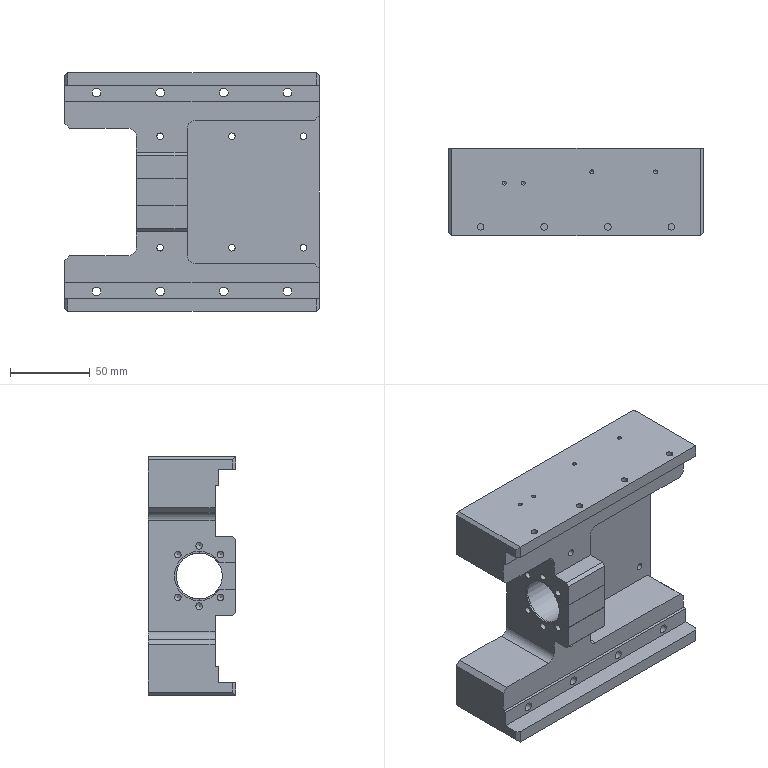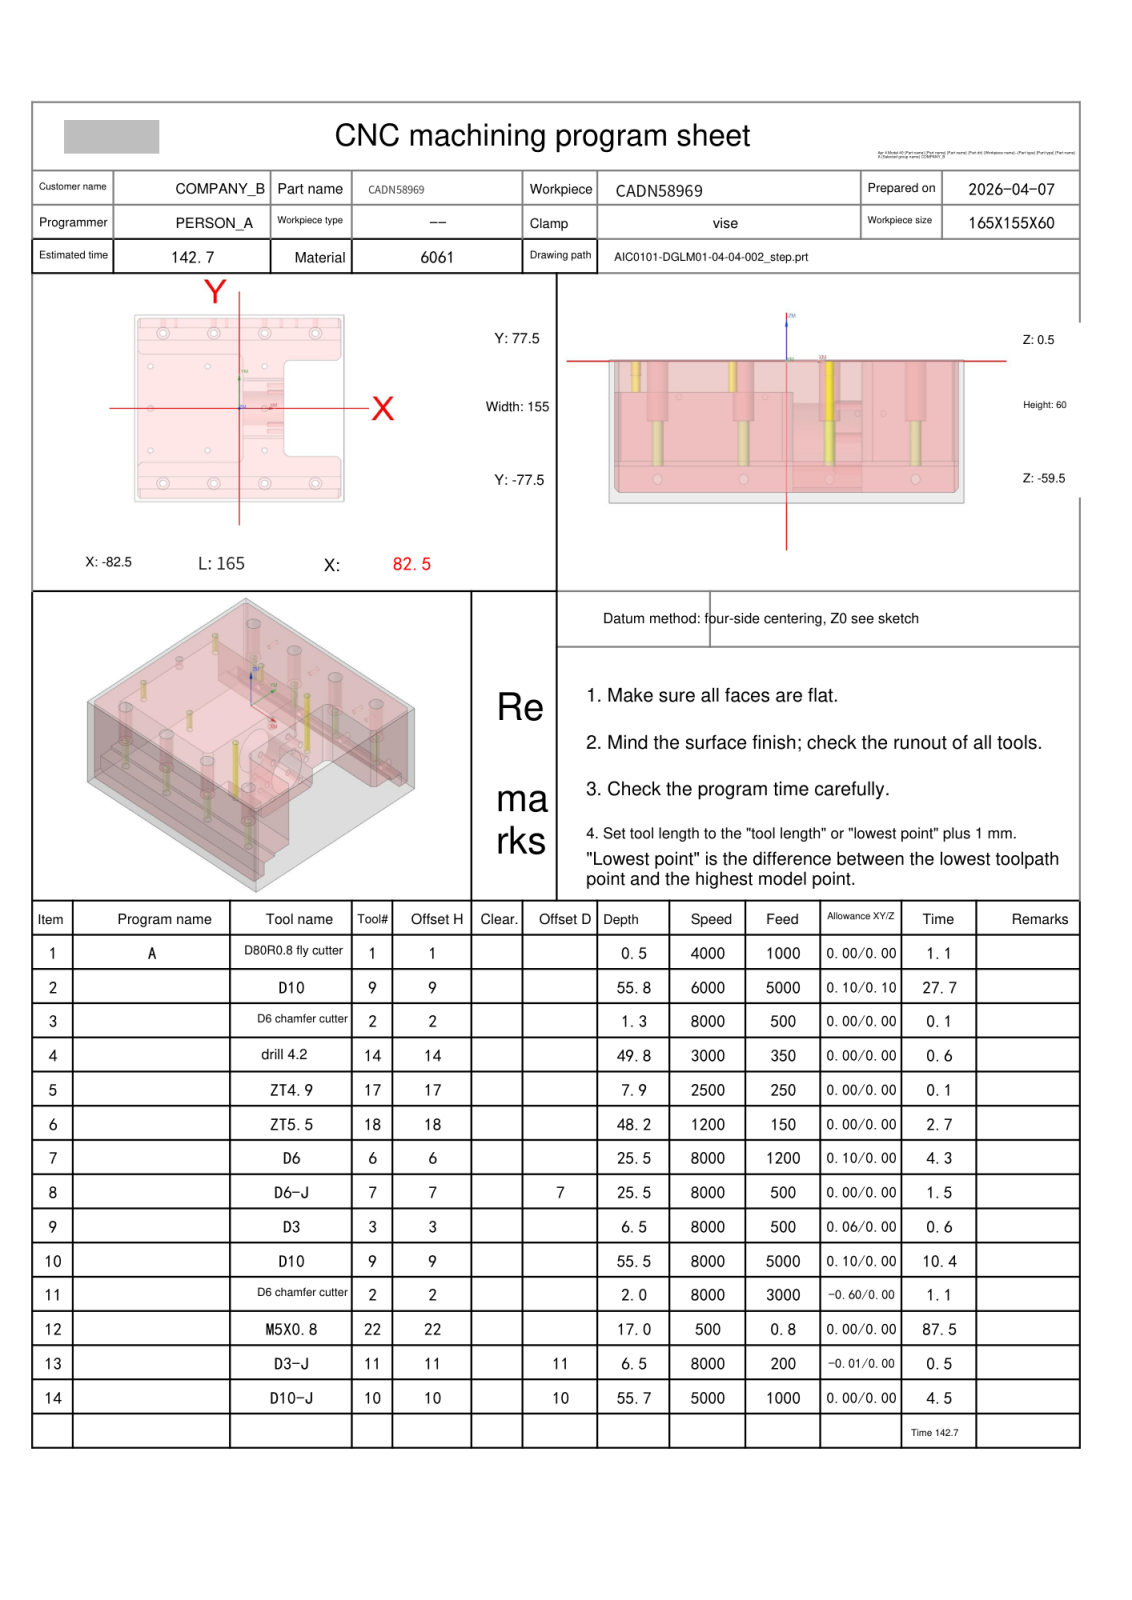NC program | NX | posted by the shop | part box 160 x 55 x 150 mm
Lines 1 to 44 of 15707:
%
O0001
(Machine time: 227.63 MIN)
(===Total Tool:12===)
(T1=D80R0.8 fly cutter D=80. R=0.8 D-H01 Z=0.    )
(T9=D10     D=10.  R=0.   D-  H09 Z=-55.3 )
(T2=D6 chamfer cutter D=6. R=0. D-H02 Z=-1.5  )
(T14=drill 4.2 D=4.2 DR_a=118 D-H14 Z=-49.26)
(T17=ZT4.9  D=4.9  DR_a=120 D-  H17 Z=-7.44 )
(T18=ZT5.5  D=5.5  DR_a=118 D-  H18 Z=-47.65)
(T6=D6      D=6.   R=0.   D-  H06 Z=-25.  )
(T7=D6-J    D=6.   R=0.   D7  H07 Z=-25.  )
(T3=D3      D=3.   R=0.   D-  H03 Z=-6.   )
(T22=M5X0.8 D=4.2  DR_a=180 D-  H22 Z=-16.5 )
(T11=D3-J   D=3.   R=0.   D11 H11 Z=-6.   )
(T10=D10-J  D=10.  R=0.   D10 H10 Z=-55.2 )
G80 G90 G17 G49 G40
G91 G28 Z0
M01
N1 T01 M06
(D80R0.8 fly cutter D=80. R=0.8 H=01 ce=0.00 di=0.00)
G00 G90 G54 X-125. Y69. M03 S4000
G43 H01 Z20.
M08
Z2.
G01 Z0.0 F1000.
X-120.
X120.
Y23.
X-120.
Y-23.
X120.
Y-69.
X-120.
X-125.
Z2.
G00 Z20.
G91 G28 Z0.0
M05
M09
G91 G28 Z0.0
M01